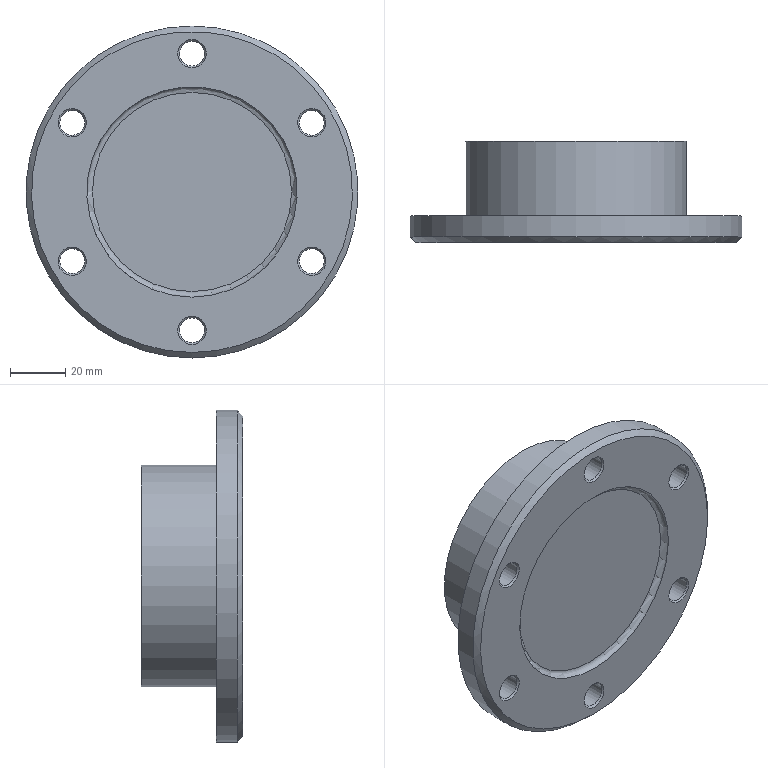Part | NX | 1 solid | 29 faces | box 120 x 36.6 x 120 mm | volume 140285 mm3 | cone 14 | cylinder 8 | plane 5 | torus 2 | commonest cylinder face diameters 9 x6 80 x1 120 x1
STEP:
#1=CARTESIAN_POINT('',(64.853,26.106,27.25));
#2=VERTEX_POINT('',#1);
#3=CARTESIAN_POINT('',(60.956,26.106,25.));
#4=DIRECTION('',(0.,-1.,0.));
#5=DIRECTION('',(0.866,0.,0.5));
#6=AXIS2_PLACEMENT_3D('',#3,#4,#5);
#7=CIRCLE('',#6,4.5);
#8=EDGE_CURVE('',#2,#2,#7,.T.);
#9=ORIENTED_EDGE('',*,*,#8,.F.);
#10=EDGE_LOOP('',(#9));
#11=FACE_BOUND('',#10,.T.);
#12=CARTESIAN_POINT('',(65.373,25.506,27.55));
#13=VERTEX_POINT('',#12);
#14=CARTESIAN_POINT('',(60.956,25.506,25.));
#15=DIRECTION('',(0.,1.,0.));
#16=DIRECTION('',(0.866,0.,0.5));
#17=AXIS2_PLACEMENT_3D('',#14,#15,#16);
#18=CIRCLE('',#17,5.1);
#19=EDGE_CURVE('',#13,#13,#18,.T.);
#20=ORIENTED_EDGE('',*,*,#19,.F.);
#21=EDGE_LOOP('',(#20));
#22=FACE_BOUND('',#21,.T.);
#23=CARTESIAN_POINT('',(60.956,25.506,25.));
#24=DIRECTION('',(0.,-1.,0.));
#25=DIRECTION('',(0.866,0.,0.5));
#26=AXIS2_PLACEMENT_3D('',#23,#24,#25);
#27=CONICAL_SURFACE('',#26,5.1,45.);
#28=ADVANCED_FACE('',(#11,#22),#27,.F.);
#29=CARTESIAN_POINT('',(57.059,34.506,22.75));
#30=VERTEX_POINT('',#29);
#31=CARTESIAN_POINT('',(60.956,34.506,25.));
#32=DIRECTION('',(0.,1.,0.));
#33=DIRECTION('',(-0.866,0.,-0.5));
#34=AXIS2_PLACEMENT_3D('',#31,#32,#33);
#35=CIRCLE('',#34,4.5);
#36=EDGE_CURVE('',#30,#30,#35,.T.);
#37=ORIENTED_EDGE('',*,*,#36,.F.);
#38=EDGE_LOOP('',(#37));
#39=FACE_BOUND('',#38,.T.);
#40=CARTESIAN_POINT('',(56.539,35.106,22.45));
#41=VERTEX_POINT('',#40);
#42=CARTESIAN_POINT('',(60.956,35.106,25.));
#43=DIRECTION('',(0.,-1.,0.));
#44=DIRECTION('',(-0.866,0.,-0.5));
#45=AXIS2_PLACEMENT_3D('',#42,#43,#44);
#46=CIRCLE('',#45,5.1);
#47=EDGE_CURVE('',#41,#41,#46,.T.);
#48=ORIENTED_EDGE('',*,*,#47,.F.);
#49=EDGE_LOOP('',(#48));
#50=FACE_BOUND('',#49,.T.);
#51=CARTESIAN_POINT('',(60.956,35.106,25.));
#52=DIRECTION('',(0.,1.,0.));
#53=DIRECTION('',(-0.866,0.,-0.5));
#54=AXIS2_PLACEMENT_3D('',#51,#52,#53);
#55=CONICAL_SURFACE('',#54,5.1,45.);
#56=ADVANCED_FACE('',(#39,#50),#55,.F.);
#57=ORIENTED_EDGE('',*,*,#36,.T.);
#58=EDGE_LOOP('',(#57));
#59=FACE_BOUND('',#58,.T.);
#60=ORIENTED_EDGE('',*,*,#8,.T.);
#61=EDGE_LOOP('',(#60));
#62=FACE_BOUND('',#61,.T.);
#63=CARTESIAN_POINT('',(60.956,25.506,25.));
#64=DIRECTION('',(0.,1.,0.));
#65=DIRECTION('',(-0.866,0.,-0.5));
#66=AXIS2_PLACEMENT_3D('',#63,#64,#65);
#67=CYLINDRICAL_SURFACE('',#66,4.5);
#68=ADVANCED_FACE('',(#59,#62),#67,.F.);
#69=CARTESIAN_POINT('',(64.853,26.106,-27.25));
#70=VERTEX_POINT('',#69);
#71=CARTESIAN_POINT('',(60.956,26.106,-25.));
#72=DIRECTION('',(0.,-1.,0.));
#73=DIRECTION('',(0.866,0.,-0.5));
#74=AXIS2_PLACEMENT_3D('',#71,#72,#73);
#75=CIRCLE('',#74,4.5);
#76=EDGE_CURVE('',#70,#70,#75,.T.);
#77=ORIENTED_EDGE('',*,*,#76,.F.);
#78=EDGE_LOOP('',(#77));
#79=FACE_BOUND('',#78,.T.);
#80=CARTESIAN_POINT('',(65.373,25.506,-27.55));
#81=VERTEX_POINT('',#80);
#82=CARTESIAN_POINT('',(60.956,25.506,-25.));
#83=DIRECTION('',(0.,1.,0.));
#84=DIRECTION('',(0.866,0.,-0.5));
#85=AXIS2_PLACEMENT_3D('',#82,#83,#84);
#86=CIRCLE('',#85,5.1);
#87=EDGE_CURVE('',#81,#81,#86,.T.);
#88=ORIENTED_EDGE('',*,*,#87,.F.);
#89=EDGE_LOOP('',(#88));
#90=FACE_BOUND('',#89,.T.);
#91=CARTESIAN_POINT('',(60.956,25.506,-25.));
#92=DIRECTION('',(0.,-1.,0.));
#93=DIRECTION('',(0.866,0.,-0.5));
#94=AXIS2_PLACEMENT_3D('',#91,#92,#93);
#95=CONICAL_SURFACE('',#94,5.1,45.);
#96=ADVANCED_FACE('',(#79,#90),#95,.F.);
#97=CARTESIAN_POINT('',(57.059,34.506,-22.75));
#98=VERTEX_POINT('',#97);
#99=CARTESIAN_POINT('',(60.956,34.506,-25.));
#100=DIRECTION('',(0.,1.,0.));
#101=DIRECTION('',(-0.866,0.,0.5));
#102=AXIS2_PLACEMENT_3D('',#99,#100,#101);
#103=CIRCLE('',#102,4.5);
#104=EDGE_CURVE('',#98,#98,#103,.T.);
#105=ORIENTED_EDGE('',*,*,#104,.F.);
#106=EDGE_LOOP('',(#105));
#107=FACE_BOUND('',#106,.T.);
#108=CARTESIAN_POINT('',(56.539,35.106,-22.45));
#109=VERTEX_POINT('',#108);
#110=CARTESIAN_POINT('',(60.956,35.106,-25.));
#111=DIRECTION('',(0.,-1.,0.));
#112=DIRECTION('',(-0.866,0.,0.5));
#113=AXIS2_PLACEMENT_3D('',#110,#111,#112);
#114=CIRCLE('',#113,5.1);
#115=EDGE_CURVE('',#109,#109,#114,.T.);
#116=ORIENTED_EDGE('',*,*,#115,.F.);
#117=EDGE_LOOP('',(#116));
#118=FACE_BOUND('',#117,.T.);
#119=CARTESIAN_POINT('',(60.956,35.106,-25.));
#120=DIRECTION('',(0.,1.,0.));
#121=DIRECTION('',(-0.866,0.,0.5));
#122=AXIS2_PLACEMENT_3D('',#119,#120,#121);
#123=CONICAL_SURFACE('',#122,5.1,45.);
#124=ADVANCED_FACE('',(#107,#118),#123,.F.);
#125=ORIENTED_EDGE('',*,*,#104,.T.);
#126=EDGE_LOOP('',(#125));
#127=FACE_BOUND('',#126,.T.);
#128=ORIENTED_EDGE('',*,*,#76,.T.);
#129=EDGE_LOOP('',(#128));
#130=FACE_BOUND('',#129,.T.);
#131=CARTESIAN_POINT('',(60.956,25.506,-25.));
#132=DIRECTION('',(0.,1.,0.));
#133=DIRECTION('',(-0.866,0.,0.5));
#134=AXIS2_PLACEMENT_3D('',#131,#132,#133);
#135=CYLINDRICAL_SURFACE('',#134,4.5);
#136=ADVANCED_FACE('',(#127,#130),#135,.F.);
#137=CARTESIAN_POINT('',(17.655,26.106,-54.5));
#138=VERTEX_POINT('',#137);
#139=CARTESIAN_POINT('',(17.655,26.106,-50.));
#140=DIRECTION('',(0.,-1.,0.));
#141=DIRECTION('',(0.,0.,-1.));
#142=AXIS2_PLACEMENT_3D('',#139,#140,#141);
#143=CIRCLE('',#142,4.5);
#144=EDGE_CURVE('',#138,#138,#143,.T.);
#145=ORIENTED_EDGE('',*,*,#144,.F.);
#146=EDGE_LOOP('',(#145));
#147=FACE_BOUND('',#146,.T.);
#148=CARTESIAN_POINT('',(17.655,25.506,-55.1));
#149=VERTEX_POINT('',#148);
#150=CARTESIAN_POINT('',(17.655,25.506,-50.));
#151=DIRECTION('',(0.,1.,0.));
#152=DIRECTION('',(0.,0.,-1.));
#153=AXIS2_PLACEMENT_3D('',#150,#151,#152);
#154=CIRCLE('',#153,5.1);
#155=EDGE_CURVE('',#149,#149,#154,.T.);
#156=ORIENTED_EDGE('',*,*,#155,.F.);
#157=EDGE_LOOP('',(#156));
#158=FACE_BOUND('',#157,.T.);
#159=CARTESIAN_POINT('',(17.655,25.506,-50.));
#160=DIRECTION('',(0.,-1.,0.));
#161=DIRECTION('',(0.,0.,-1.));
#162=AXIS2_PLACEMENT_3D('',#159,#160,#161);
#163=CONICAL_SURFACE('',#162,5.1,45.);
#164=ADVANCED_FACE('',(#147,#158),#163,.F.);
#165=CARTESIAN_POINT('',(17.655,34.506,-45.5));
#166=VERTEX_POINT('',#165);
#167=CARTESIAN_POINT('',(17.655,34.506,-50.));
#168=DIRECTION('',(0.,1.,0.));
#169=DIRECTION('',(0.,0.,1.));
#170=AXIS2_PLACEMENT_3D('',#167,#168,#169);
#171=CIRCLE('',#170,4.5);
#172=EDGE_CURVE('',#166,#166,#171,.T.);
#173=ORIENTED_EDGE('',*,*,#172,.F.);
#174=EDGE_LOOP('',(#173));
#175=FACE_BOUND('',#174,.T.);
#176=CARTESIAN_POINT('',(17.655,35.106,-44.9));
#177=VERTEX_POINT('',#176);
#178=CARTESIAN_POINT('',(17.655,35.106,-50.));
#179=DIRECTION('',(0.,-1.,0.));
#180=DIRECTION('',(0.,0.,1.));
#181=AXIS2_PLACEMENT_3D('',#178,#179,#180);
#182=CIRCLE('',#181,5.1);
#183=EDGE_CURVE('',#177,#177,#182,.T.);
#184=ORIENTED_EDGE('',*,*,#183,.F.);
#185=EDGE_LOOP('',(#184));
#186=FACE_BOUND('',#185,.T.);
#187=CARTESIAN_POINT('',(17.655,35.106,-50.));
#188=DIRECTION('',(0.,1.,0.));
#189=DIRECTION('',(0.,0.,1.));
#190=AXIS2_PLACEMENT_3D('',#187,#188,#189);
#191=CONICAL_SURFACE('',#190,5.1,45.);
#192=ADVANCED_FACE('',(#175,#186),#191,.F.);
#193=ORIENTED_EDGE('',*,*,#172,.T.);
#194=EDGE_LOOP('',(#193));
#195=FACE_BOUND('',#194,.T.);
#196=ORIENTED_EDGE('',*,*,#144,.T.);
#197=EDGE_LOOP('',(#196));
#198=FACE_BOUND('',#197,.T.);
#199=CARTESIAN_POINT('',(17.655,25.506,-50.));
#200=DIRECTION('',(0.,1.,0.));
#201=DIRECTION('',(0.,0.,1.));
#202=AXIS2_PLACEMENT_3D('',#199,#200,#201);
#203=CYLINDRICAL_SURFACE('',#202,4.5);
#204=ADVANCED_FACE('',(#195,#198),#203,.F.);
#205=CARTESIAN_POINT('',(-29.544,26.106,-27.25));
#206=VERTEX_POINT('',#205);
#207=CARTESIAN_POINT('',(-25.647,26.106,-25.));
#208=DIRECTION('',(0.,-1.,0.));
#209=DIRECTION('',(-0.866,0.,-0.5));
#210=AXIS2_PLACEMENT_3D('',#207,#208,#209);
#211=CIRCLE('',#210,4.5);
#212=EDGE_CURVE('',#206,#206,#211,.T.);
#213=ORIENTED_EDGE('',*,*,#212,.F.);
#214=EDGE_LOOP('',(#213));
#215=FACE_BOUND('',#214,.T.);
#216=CARTESIAN_POINT('',(-30.063,25.506,-27.55));
#217=VERTEX_POINT('',#216);
#218=CARTESIAN_POINT('',(-25.647,25.506,-25.));
#219=DIRECTION('',(0.,1.,0.));
#220=DIRECTION('',(-0.866,0.,-0.5));
#221=AXIS2_PLACEMENT_3D('',#218,#219,#220);
#222=CIRCLE('',#221,5.1);
#223=EDGE_CURVE('',#217,#217,#222,.T.);
#224=ORIENTED_EDGE('',*,*,#223,.F.);
#225=EDGE_LOOP('',(#224));
#226=FACE_BOUND('',#225,.T.);
#227=CARTESIAN_POINT('',(-25.647,25.506,-25.));
#228=DIRECTION('',(0.,-1.,0.));
#229=DIRECTION('',(-0.866,0.,-0.5));
#230=AXIS2_PLACEMENT_3D('',#227,#228,#229);
#231=CONICAL_SURFACE('',#230,5.1,45.);
#232=ADVANCED_FACE('',(#215,#226),#231,.F.);
#233=CARTESIAN_POINT('',(-21.75,34.506,-22.75));
#234=VERTEX_POINT('',#233);
#235=CARTESIAN_POINT('',(-25.647,34.506,-25.));
#236=DIRECTION('',(0.,1.,0.));
#237=DIRECTION('',(0.866,0.,0.5));
#238=AXIS2_PLACEMENT_3D('',#235,#236,#237);
#239=CIRCLE('',#238,4.5);
#240=EDGE_CURVE('',#234,#234,#239,.T.);
#241=ORIENTED_EDGE('',*,*,#240,.F.);
#242=EDGE_LOOP('',(#241));
#243=FACE_BOUND('',#242,.T.);
#244=CARTESIAN_POINT('',(-21.23,35.106,-22.45));
#245=VERTEX_POINT('',#244);
#246=CARTESIAN_POINT('',(-25.647,35.106,-25.));
#247=DIRECTION('',(0.,-1.,0.));
#248=DIRECTION('',(0.866,0.,0.5));
#249=AXIS2_PLACEMENT_3D('',#246,#247,#248);
#250=CIRCLE('',#249,5.1);
#251=EDGE_CURVE('',#245,#245,#250,.T.);
#252=ORIENTED_EDGE('',*,*,#251,.F.);
#253=EDGE_LOOP('',(#252));
#254=FACE_BOUND('',#253,.T.);
#255=CARTESIAN_POINT('',(-25.647,35.106,-25.));
#256=DIRECTION('',(0.,1.,0.));
#257=DIRECTION('',(0.866,0.,0.5));
#258=AXIS2_PLACEMENT_3D('',#255,#256,#257);
#259=CONICAL_SURFACE('',#258,5.1,45.);
#260=ADVANCED_FACE('',(#243,#254),#259,.F.);
#261=ORIENTED_EDGE('',*,*,#240,.T.);
#262=EDGE_LOOP('',(#261));
#263=FACE_BOUND('',#262,.T.);
#264=ORIENTED_EDGE('',*,*,#212,.T.);
#265=EDGE_LOOP('',(#264));
#266=FACE_BOUND('',#265,.T.);
#267=CARTESIAN_POINT('',(-25.647,25.506,-25.));
#268=DIRECTION('',(0.,1.,0.));
#269=DIRECTION('',(0.866,0.,0.5));
#270=AXIS2_PLACEMENT_3D('',#267,#268,#269);
#271=CYLINDRICAL_SURFACE('',#270,4.5);
#272=ADVANCED_FACE('',(#263,#266),#271,.F.);
#273=CARTESIAN_POINT('',(-29.544,26.106,27.25));
#274=VERTEX_POINT('',#273);
#275=CARTESIAN_POINT('',(-25.647,26.106,25.));
#276=DIRECTION('',(0.,-1.,0.));
#277=DIRECTION('',(-0.866,0.,0.5));
#278=AXIS2_PLACEMENT_3D('',#275,#276,#277);
#279=CIRCLE('',#278,4.5);
#280=EDGE_CURVE('',#274,#274,#279,.T.);
#281=ORIENTED_EDGE('',*,*,#280,.F.);
#282=EDGE_LOOP('',(#281));
#283=FACE_BOUND('',#282,.T.);
#284=CARTESIAN_POINT('',(-30.063,25.506,27.55));
#285=VERTEX_POINT('',#284);
#286=CARTESIAN_POINT('',(-25.647,25.506,25.));
#287=DIRECTION('',(0.,1.,0.));
#288=DIRECTION('',(-0.866,0.,0.5));
#289=AXIS2_PLACEMENT_3D('',#286,#287,#288);
#290=CIRCLE('',#289,5.1);
#291=EDGE_CURVE('',#285,#285,#290,.T.);
#292=ORIENTED_EDGE('',*,*,#291,.F.);
#293=EDGE_LOOP('',(#292));
#294=FACE_BOUND('',#293,.T.);
#295=CARTESIAN_POINT('',(-25.647,25.506,25.));
#296=DIRECTION('',(0.,-1.,0.));
#297=DIRECTION('',(-0.866,0.,0.5));
#298=AXIS2_PLACEMENT_3D('',#295,#296,#297);
#299=CONICAL_SURFACE('',#298,5.1,45.);
#300=ADVANCED_FACE('',(#283,#294),#299,.F.);
#301=CARTESIAN_POINT('',(-21.75,34.506,22.75));
#302=VERTEX_POINT('',#301);
#303=CARTESIAN_POINT('',(-25.647,34.506,25.));
#304=DIRECTION('',(0.,1.,0.));
#305=DIRECTION('',(0.866,0.,-0.5));
#306=AXIS2_PLACEMENT_3D('',#303,#304,#305);
#307=CIRCLE('',#306,4.5);
#308=EDGE_CURVE('',#302,#302,#307,.T.);
#309=ORIENTED_EDGE('',*,*,#308,.F.);
#310=EDGE_LOOP('',(#309));
#311=FACE_BOUND('',#310,.T.);
#312=CARTESIAN_POINT('',(-21.23,35.106,22.45));
#313=VERTEX_POINT('',#312);
#314=CARTESIAN_POINT('',(-25.647,35.106,25.));
#315=DIRECTION('',(0.,-1.,0.));
#316=DIRECTION('',(0.866,0.,-0.5));
#317=AXIS2_PLACEMENT_3D('',#314,#315,#316);
#318=CIRCLE('',#317,5.1);
#319=EDGE_CURVE('',#313,#313,#318,.T.);
#320=ORIENTED_EDGE('',*,*,#319,.F.);
#321=EDGE_LOOP('',(#320));
#322=FACE_BOUND('',#321,.T.);
#323=CARTESIAN_POINT('',(-25.647,35.106,25.));
#324=DIRECTION('',(0.,1.,0.));
#325=DIRECTION('',(0.866,0.,-0.5));
#326=AXIS2_PLACEMENT_3D('',#323,#324,#325);
#327=CONICAL_SURFACE('',#326,5.1,45.);
#328=ADVANCED_FACE('',(#311,#322),#327,.F.);
#329=ORIENTED_EDGE('',*,*,#308,.T.);
#330=EDGE_LOOP('',(#329));
#331=FACE_BOUND('',#330,.T.);
#332=ORIENTED_EDGE('',*,*,#280,.T.);
#333=EDGE_LOOP('',(#332));
#334=FACE_BOUND('',#333,.T.);
#335=CARTESIAN_POINT('',(-25.647,25.506,25.));
#336=DIRECTION('',(0.,1.,0.));
#337=DIRECTION('',(0.866,0.,-0.5));
#338=AXIS2_PLACEMENT_3D('',#335,#336,#337);
#339=CYLINDRICAL_SURFACE('',#338,4.5);
#340=ADVANCED_FACE('',(#331,#334),#339,.F.);
#341=CARTESIAN_POINT('',(17.655,27.506,-36.));
#342=VERTEX_POINT('',#341);
#343=CARTESIAN_POINT('',(17.655,27.506,0.));
#344=DIRECTION('',(0.,-1.,0.));
#345=DIRECTION('',(0.,0.,-1.));
#346=AXIS2_PLACEMENT_3D('',#343,#344,#345);
#347=CIRCLE('',#346,36.);
#348=EDGE_CURVE('',#342,#342,#347,.T.);
#349=ORIENTED_EDGE('',*,*,#348,.T.);
#350=EDGE_LOOP('',(#349));
#351=FACE_OUTER_BOUND('',#350,.T.);
#352=CARTESIAN_POINT('',(-18.345,27.506,0.));
#353=DIRECTION('',(0.,1.,0.));
#354=DIRECTION('',(0.,0.,-1.));
#355=AXIS2_PLACEMENT_3D('',#352,#353,#354);
#356=PLANE('',#355);
#357=ADVANCED_FACE('',(#351),#356,.F.);
#358=ORIENTED_EDGE('',*,*,#348,.F.);
#359=EDGE_LOOP('',(#358));
#360=FACE_BOUND('',#359,.T.);
#361=CARTESIAN_POINT('',(17.655,25.506,-38.));
#362=VERTEX_POINT('',#361);
#363=CARTESIAN_POINT('',(17.655,25.506,0.));
#364=DIRECTION('',(0.,-1.,0.));
#365=DIRECTION('',(0.,0.,-1.));
#366=AXIS2_PLACEMENT_3D('',#363,#364,#365);
#367=CIRCLE('',#366,38.);
#368=EDGE_CURVE('',#362,#362,#367,.T.);
#369=ORIENTED_EDGE('',*,*,#368,.T.);
#370=EDGE_LOOP('',(#369));
#371=FACE_BOUND('',#370,.T.);
#372=CARTESIAN_POINT('',(17.655,25.506,0.));
#373=DIRECTION('',(0.,-1.,0.));
#374=DIRECTION('',(0.,0.,1.));
#375=AXIS2_PLACEMENT_3D('',#372,#373,#374);
#376=TOROIDAL_SURFACE('',#375,36.,2.);
#377=ADVANCED_FACE('',(#360,#371),#376,.F.);
#378=ORIENTED_EDGE('',*,*,#19,.T.);
#379=EDGE_LOOP('',(#378));
#380=FACE_BOUND('',#379,.T.);
#381=ORIENTED_EDGE('',*,*,#87,.T.);
#382=EDGE_LOOP('',(#381));
#383=FACE_BOUND('',#382,.T.);
#384=ORIENTED_EDGE('',*,*,#155,.T.);
#385=EDGE_LOOP('',(#384));
#386=FACE_BOUND('',#385,.T.);
#387=ORIENTED_EDGE('',*,*,#223,.T.);
#388=EDGE_LOOP('',(#387));
#389=FACE_BOUND('',#388,.T.);
#390=ORIENTED_EDGE('',*,*,#291,.T.);
#391=EDGE_LOOP('',(#390));
#392=FACE_BOUND('',#391,.T.);
#393=CARTESIAN_POINT('',(17.655,25.506,55.1));
#394=VERTEX_POINT('',#393);
#395=CARTESIAN_POINT('',(17.655,25.506,50.));
#396=DIRECTION('',(0.,1.,0.));
#397=DIRECTION('',(0.,0.,1.));
#398=AXIS2_PLACEMENT_3D('',#395,#396,#397);
#399=CIRCLE('',#398,5.1);
#400=EDGE_CURVE('',#394,#394,#399,.T.);
#401=ORIENTED_EDGE('',*,*,#400,.T.);
#402=EDGE_LOOP('',(#401));
#403=FACE_BOUND('',#402,.T.);
#404=ORIENTED_EDGE('',*,*,#368,.F.);
#405=EDGE_LOOP('',(#404));
#406=FACE_BOUND('',#405,.T.);
#407=CARTESIAN_POINT('',(17.655,25.506,-58.));
#408=VERTEX_POINT('',#407);
#409=CARTESIAN_POINT('',(17.655,25.506,0.));
#410=DIRECTION('',(0.,-1.,0.));
#411=DIRECTION('',(0.,0.,-1.));
#412=AXIS2_PLACEMENT_3D('',#409,#410,#411);
#413=CIRCLE('',#412,58.);
#414=EDGE_CURVE('',#408,#408,#413,.T.);
#415=ORIENTED_EDGE('',*,*,#414,.T.);
#416=EDGE_LOOP('',(#415));
#417=FACE_BOUND('',#416,.T.);
#418=CARTESIAN_POINT('',(-40.345,25.506,0.));
#419=DIRECTION('',(0.,1.,0.));
#420=DIRECTION('',(0.,0.,-1.));
#421=AXIS2_PLACEMENT_3D('',#418,#419,#420);
#422=PLANE('',#421);
#423=ADVANCED_FACE('',(#380,#383,#386,#389,#392,#403,#406,#417),#422,.F.);
#424=ORIENTED_EDGE('',*,*,#414,.F.);
#425=EDGE_LOOP('',(#424));
#426=FACE_BOUND('',#425,.T.);
#427=CARTESIAN_POINT('',(17.655,27.506,-60.));
#428=VERTEX_POINT('',#427);
#429=CARTESIAN_POINT('',(17.655,27.506,0.));
#430=DIRECTION('',(0.,-1.,0.));
#431=DIRECTION('',(0.,0.,-1.));
#432=AXIS2_PLACEMENT_3D('',#429,#430,#431);
#433=CIRCLE('',#432,60.);
#434=EDGE_CURVE('',#428,#428,#433,.T.);
#435=ORIENTED_EDGE('',*,*,#434,.T.);
#436=EDGE_LOOP('',(#435));
#437=FACE_BOUND('',#436,.T.);
#438=CARTESIAN_POINT('',(17.655,27.506,0.));
#439=DIRECTION('',(0.,1.,0.));
#440=DIRECTION('',(0.,0.,-1.));
#441=AXIS2_PLACEMENT_3D('',#438,#439,#440);
#442=CONICAL_SURFACE('',#441,60.,45.);
#443=ADVANCED_FACE('',(#426,#437),#442,.T.);
#444=ORIENTED_EDGE('',*,*,#434,.F.);
#445=EDGE_LOOP('',(#444));
#446=FACE_BOUND('',#445,.T.);
#447=CARTESIAN_POINT('',(17.655,35.106,-60.));
#448=VERTEX_POINT('',#447);
#449=CARTESIAN_POINT('',(17.655,35.106,0.));
#450=DIRECTION('',(0.,-1.,0.));
#451=DIRECTION('',(0.,0.,-1.));
#452=AXIS2_PLACEMENT_3D('',#449,#450,#451);
#453=CIRCLE('',#452,60.);
#454=EDGE_CURVE('',#448,#448,#453,.T.);
#455=ORIENTED_EDGE('',*,*,#454,.T.);
#456=EDGE_LOOP('',(#455));
#457=FACE_BOUND('',#456,.T.);
#458=CARTESIAN_POINT('',(17.655,14.806,0.));
#459=DIRECTION('',(0.,-1.,0.));
#460=DIRECTION('',(0.,0.,1.));
#461=AXIS2_PLACEMENT_3D('',#458,#459,#460);
#462=CYLINDRICAL_SURFACE('',#461,60.);
#463=ADVANCED_FACE('',(#446,#457),#462,.T.);
#464=ORIENTED_EDGE('',*,*,#47,.T.);
#465=EDGE_LOOP('',(#464));
#466=FACE_BOUND('',#465,.T.);
#467=ORIENTED_EDGE('',*,*,#115,.T.);
#468=EDGE_LOOP('',(#467));
#469=FACE_BOUND('',#468,.T.);
#470=ORIENTED_EDGE('',*,*,#183,.T.);
#471=EDGE_LOOP('',(#470));
#472=FACE_BOUND('',#471,.T.);
#473=ORIENTED_EDGE('',*,*,#251,.T.);
#474=EDGE_LOOP('',(#473));
#475=FACE_BOUND('',#474,.T.);
#476=ORIENTED_EDGE('',*,*,#319,.T.);
#477=EDGE_LOOP('',(#476));
#478=FACE_BOUND('',#477,.T.);
#479=CARTESIAN_POINT('',(17.655,35.106,44.9));
#480=VERTEX_POINT('',#479);
#481=CARTESIAN_POINT('',(17.655,35.106,50.));
#482=DIRECTION('',(0.,-1.,0.));
#483=DIRECTION('',(0.,0.,-1.));
#484=AXIS2_PLACEMENT_3D('',#481,#482,#483);
#485=CIRCLE('',#484,5.1);
#486=EDGE_CURVE('',#480,#480,#485,.T.);
#487=ORIENTED_EDGE('',*,*,#486,.T.);
#488=EDGE_LOOP('',(#487));
#489=FACE_BOUND('',#488,.T.);
#490=ORIENTED_EDGE('',*,*,#454,.F.);
#491=EDGE_LOOP('',(#490));
#492=FACE_BOUND('',#491,.T.);
#493=CARTESIAN_POINT('',(17.655,35.106,-40.));
#494=VERTEX_POINT('',#493);
#495=CARTESIAN_POINT('',(17.655,35.106,0.));
#496=DIRECTION('',(0.,-1.,0.));
#497=DIRECTION('',(0.,0.,-1.));
#498=AXIS2_PLACEMENT_3D('',#495,#496,#497);
#499=CIRCLE('',#498,40.);
#500=EDGE_CURVE('',#494,#494,#499,.T.);
#501=ORIENTED_EDGE('',*,*,#500,.T.);
#502=EDGE_LOOP('',(#501));
#503=FACE_BOUND('',#502,.T.);
#504=CARTESIAN_POINT('',(-22.345,35.106,0.));
#505=DIRECTION('',(0.,-1.,0.));
#506=DIRECTION('',(0.,0.,1.));
#507=AXIS2_PLACEMENT_3D('',#504,#505,#506);
#508=PLANE('',#507);
#509=ADVANCED_FACE('',(#466,#469,#472,#475,#478,#489,#492,#503),#508,.F.);
#510=ORIENTED_EDGE('',*,*,#500,.F.);
#511=EDGE_LOOP('',(#510));
#512=FACE_BOUND('',#511,.T.);
#513=CARTESIAN_POINT('',(17.655,62.106,-40.));
#514=VERTEX_POINT('',#513);
#515=CARTESIAN_POINT('',(17.655,62.106,0.));
#516=DIRECTION('',(0.,-1.,0.));
#517=DIRECTION('',(0.,0.,-1.));
#518=AXIS2_PLACEMENT_3D('',#515,#516,#517);
#519=CIRCLE('',#518,40.);
#520=EDGE_CURVE('',#514,#514,#519,.T.);
#521=ORIENTED_EDGE('',*,*,#520,.T.);
#522=EDGE_LOOP('',(#521));
#523=FACE_BOUND('',#522,.T.);
#524=CARTESIAN_POINT('',(17.655,14.806,0.));
#525=DIRECTION('',(0.,-1.,0.));
#526=DIRECTION('',(0.,0.,1.));
#527=AXIS2_PLACEMENT_3D('',#524,#525,#526);
#528=CYLINDRICAL_SURFACE('',#527,40.);
#529=ADVANCED_FACE('',(#512,#523),#528,.T.);
#530=ORIENTED_EDGE('',*,*,#520,.F.);
#531=EDGE_LOOP('',(#530));
#532=FACE_BOUND('',#531,.T.);
#533=CARTESIAN_POINT('',(17.655,62.106,-36.5));
#534=VERTEX_POINT('',#533);
#535=CARTESIAN_POINT('',(17.655,62.106,0.));
#536=DIRECTION('',(0.,-1.,0.));
#537=DIRECTION('',(0.,0.,-1.));
#538=AXIS2_PLACEMENT_3D('',#535,#536,#537);
#539=CIRCLE('',#538,36.5);
#540=EDGE_CURVE('',#534,#534,#539,.T.);
#541=ORIENTED_EDGE('',*,*,#540,.T.);
#542=EDGE_LOOP('',(#541));
#543=FACE_BOUND('',#542,.T.);
#544=CARTESIAN_POINT('',(-18.845,62.106,0.));
#545=DIRECTION('',(0.,-1.,0.));
#546=DIRECTION('',(0.,0.,1.));
#547=AXIS2_PLACEMENT_3D('',#544,#545,#546);
#548=PLANE('',#547);
#549=ADVANCED_FACE('',(#532,#543),#548,.F.);
#550=ORIENTED_EDGE('',*,*,#540,.F.);
#551=EDGE_LOOP('',(#550));
#552=FACE_BOUND('',#551,.T.);
#553=CARTESIAN_POINT('',(17.655,44.257,-35.608));
#554=VERTEX_POINT('',#553);
#555=CARTESIAN_POINT('',(17.655,44.257,0.));
#556=DIRECTION('',(0.,-1.,0.));
#557=DIRECTION('',(0.,0.,-1.));
#558=AXIS2_PLACEMENT_3D('',#555,#556,#557);
#559=CIRCLE('',#558,35.608);
#560=EDGE_CURVE('',#554,#554,#559,.T.);
#561=ORIENTED_EDGE('',*,*,#560,.T.);
#562=EDGE_LOOP('',(#561));
#563=FACE_BOUND('',#562,.T.);
#564=CARTESIAN_POINT('',(17.655,44.257,0.));
#565=DIRECTION('',(0.,1.,0.));
#566=DIRECTION('',(0.,0.,-1.));
#567=AXIS2_PLACEMENT_3D('',#564,#565,#566);
#568=CONICAL_SURFACE('',#567,35.608,2.862);
#569=ADVANCED_FACE('',(#552,#563),#568,.F.);
#570=ORIENTED_EDGE('',*,*,#560,.F.);
#571=EDGE_LOOP('',(#570));
#572=FACE_BOUND('',#571,.T.);
#573=CARTESIAN_POINT('',(17.655,39.506,-30.614));
#574=VERTEX_POINT('',#573);
#575=CARTESIAN_POINT('',(17.655,39.506,0.));
#576=DIRECTION('',(0.,-1.,0.));
#577=DIRECTION('',(0.,0.,-1.));
#578=AXIS2_PLACEMENT_3D('',#575,#576,#577);
#579=CIRCLE('',#578,30.614);
#580=EDGE_CURVE('',#574,#574,#579,.T.);
#581=ORIENTED_EDGE('',*,*,#580,.T.);
#582=EDGE_LOOP('',(#581));
#583=FACE_BOUND('',#582,.T.);
#584=CARTESIAN_POINT('',(17.655,44.506,0.));
#585=DIRECTION('',(0.,-1.,0.));
#586=DIRECTION('',(0.,0.,1.));
#587=AXIS2_PLACEMENT_3D('',#584,#585,#586);
#588=TOROIDAL_SURFACE('',#587,30.614,5.);
#589=ADVANCED_FACE('',(#572,#583),#588,.F.);
#590=ORIENTED_EDGE('',*,*,#580,.F.);
#591=EDGE_LOOP('',(#590));
#592=FACE_OUTER_BOUND('',#591,.T.);
#593=CARTESIAN_POINT('',(17.655,39.506,0.));
#594=DIRECTION('',(0.,-1.,0.));
#595=DIRECTION('',(0.,0.,1.));
#596=AXIS2_PLACEMENT_3D('',#593,#594,#595);
#597=PLANE('',#596);
#598=ADVANCED_FACE('',(#592),#597,.F.);
#599=CARTESIAN_POINT('',(17.655,34.506,45.5));
#600=VERTEX_POINT('',#599);
#601=CARTESIAN_POINT('',(17.655,34.506,50.));
#602=DIRECTION('',(0.,1.,0.));
#603=DIRECTION('',(0.,0.,-1.));
#604=AXIS2_PLACEMENT_3D('',#601,#602,#603);
#605=CIRCLE('',#604,4.5);
#606=EDGE_CURVE('',#600,#600,#605,.T.);
#607=ORIENTED_EDGE('',*,*,#606,.T.);
#608=EDGE_LOOP('',(#607));
#609=FACE_BOUND('',#608,.T.);
#610=CARTESIAN_POINT('',(17.655,26.106,54.5));
#611=VERTEX_POINT('',#610);
#612=CARTESIAN_POINT('',(17.655,26.106,50.));
#613=DIRECTION('',(0.,-1.,0.));
#614=DIRECTION('',(0.,0.,1.));
#615=AXIS2_PLACEMENT_3D('',#612,#613,#614);
#616=CIRCLE('',#615,4.5);
#617=EDGE_CURVE('',#611,#611,#616,.T.);
#618=ORIENTED_EDGE('',*,*,#617,.T.);
#619=EDGE_LOOP('',(#618));
#620=FACE_BOUND('',#619,.T.);
#621=CARTESIAN_POINT('',(17.655,25.506,50.));
#622=DIRECTION('',(0.,1.,0.));
#623=DIRECTION('',(0.,0.,-1.));
#624=AXIS2_PLACEMENT_3D('',#621,#622,#623);
#625=CYLINDRICAL_SURFACE('',#624,4.5);
#626=ADVANCED_FACE('',(#609,#620),#625,.F.);
#627=ORIENTED_EDGE('',*,*,#617,.F.);
#628=EDGE_LOOP('',(#627));
#629=FACE_BOUND('',#628,.T.);
#630=ORIENTED_EDGE('',*,*,#400,.F.);
#631=EDGE_LOOP('',(#630));
#632=FACE_BOUND('',#631,.T.);
#633=CARTESIAN_POINT('',(17.655,25.506,50.));
#634=DIRECTION('',(0.,-1.,0.));
#635=DIRECTION('',(0.,0.,1.));
#636=AXIS2_PLACEMENT_3D('',#633,#634,#635);
#637=CONICAL_SURFACE('',#636,5.1,45.);
#638=ADVANCED_FACE('',(#629,#632),#637,.F.);
#639=ORIENTED_EDGE('',*,*,#606,.F.);
#640=EDGE_LOOP('',(#639));
#641=FACE_BOUND('',#640,.T.);
#642=ORIENTED_EDGE('',*,*,#486,.F.);
#643=EDGE_LOOP('',(#642));
#644=FACE_BOUND('',#643,.T.);
#645=CARTESIAN_POINT('',(17.655,35.106,50.));
#646=DIRECTION('',(0.,1.,0.));
#647=DIRECTION('',(0.,0.,-1.));
#648=AXIS2_PLACEMENT_3D('',#645,#646,#647);
#649=CONICAL_SURFACE('',#648,5.1,45.);
#650=ADVANCED_FACE('',(#641,#644),#649,.F.);
#651=CLOSED_SHELL('',(#28,#56,#68,#96,#124,#136,#164,#192,#204,#232,#260,#272,#300,#328,#340,#357,#377,#423,#443,#463,#509,#529,#549,#569,#589,#598,#626,#638,#650));
#652=MANIFOLD_SOLID_BREP('',#651);
#653=(LENGTH_UNIT()NAMED_UNIT(*)SI_UNIT(.MILLI.,.METRE.));
#654=UNCERTAINTY_MEASURE_WITH_UNIT(LENGTH_MEASURE(0.00002),#653,'','');
#655=(NAMED_UNIT(*)PLANE_ANGLE_UNIT()SI_UNIT($,.RADIAN.));
#656=PLANE_ANGLE_MEASURE_WITH_UNIT(PLANE_ANGLE_MEASURE(0.01745),#655);
#657=DIMENSIONAL_EXPONENTS(0.,0.,0.,0.,0.,0.,0.);
#658=(CONVERSION_BASED_UNIT('DEGREE',#656)NAMED_UNIT(#657)PLANE_ANGLE_UNIT());
#659=(NAMED_UNIT(*)SI_UNIT($,.STERADIAN.)SOLID_ANGLE_UNIT());
#660=(GEOMETRIC_REPRESENTATION_CONTEXT(3)GLOBAL_UNCERTAINTY_ASSIGNED_CONTEXT((#654))GLOBAL_UNIT_ASSIGNED_CONTEXT((#653,#658,#659))REPRESENTATION_CONTEXT('',''));
#661=ADVANCED_BREP_SHAPE_REPRESENTATION('',(#652),#660);